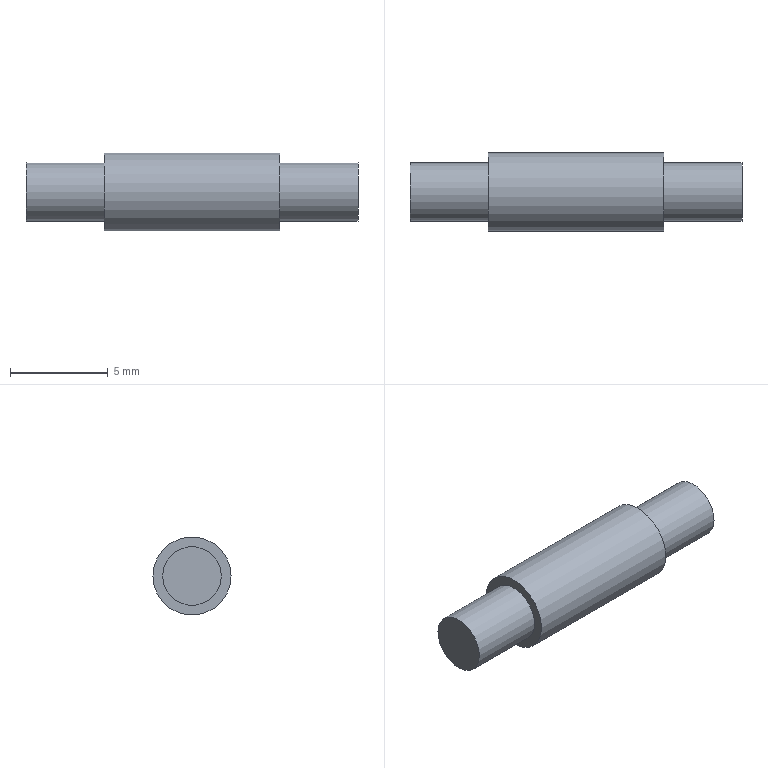Part | STEP file | 2-11.4 | 1 solid | 7 faces | box 17 x 4 x 4 mm | volume 169.646 mm3 | plane 4 | cylinder 3 | commonest cylinder face diameters 3 x2 4 x1
STEP:
#1=CARTESIAN_POINT('',(0.,0.,0.));
#2=DIRECTION('',(0.,0.,1.));
#3=DIRECTION('',(1.,0.,0.));
#4=AXIS2_PLACEMENT_3D('',#1,#2,#3);
#5=CARTESIAN_POINT('',(4.5,2.,0.));
#6=VERTEX_POINT('',#5);
#7=CARTESIAN_POINT('',(-4.5,2.,0.));
#8=VERTEX_POINT('',#7);
#9=CARTESIAN_POINT('',(4.5,2.,0.));
#10=DIRECTION('',(-1.,0.,0.));
#11=VECTOR('',#10,1.);
#12=LINE('',#9,#11);
#13=CARTESIAN_POINT('',(4.5,0.,0.));
#14=DIRECTION('',(-1.,0.,0.));
#15=DIRECTION('',(0.,1.,0.));
#16=AXIS2_PLACEMENT_3D('',#13,#14,#15);
#17=CYLINDRICAL_SURFACE('',#16,2.);
#18=CARTESIAN_POINT('',(6.283,0.));
#19=DIRECTION('',(0.,1.));
#20=VECTOR('',#19,1.);
#21=LINE('',#18,#20);
#22=(GEOMETRIC_REPRESENTATION_CONTEXT(2)PARAMETRIC_REPRESENTATION_CONTEXT()REPRESENTATION_CONTEXT('',''));
#23=DEFINITIONAL_REPRESENTATION('',(#21),#22);
#24=PCURVE('',#17,#23);
#25=CARTESIAN_POINT('',(0.,0.));
#26=DIRECTION('',(0.,1.));
#27=VECTOR('',#26,1.);
#28=LINE('',#25,#27);
#29=(GEOMETRIC_REPRESENTATION_CONTEXT(2)PARAMETRIC_REPRESENTATION_CONTEXT()REPRESENTATION_CONTEXT('',''));
#30=DEFINITIONAL_REPRESENTATION('',(#28),#29);
#31=PCURVE('',#17,#30);
#32=SEAM_CURVE('',#12,(#24,#31),.PCURVE_S1.);
#33=EDGE_CURVE('',#6,#8,#32,.T.);
#34=ORIENTED_EDGE('',*,*,#33,.T.);
#35=CARTESIAN_POINT('',(-4.5,0.,0.));
#36=DIRECTION('',(1.,0.,0.));
#37=DIRECTION('',(0.,1.,0.));
#38=AXIS2_PLACEMENT_3D('',#35,#36,#37);
#39=CIRCLE('',#38,2.);
#40=CARTESIAN_POINT('',(6.283,9.));
#41=DIRECTION('',(-1.,0.));
#42=VECTOR('',#41,1.);
#43=LINE('',#40,#42);
#44=(GEOMETRIC_REPRESENTATION_CONTEXT(2)PARAMETRIC_REPRESENTATION_CONTEXT()REPRESENTATION_CONTEXT('',''));
#45=DEFINITIONAL_REPRESENTATION('',(#43),#44);
#46=PCURVE('',#17,#45);
#47=CARTESIAN_POINT('',(-4.5,-0.5359,0.));
#48=DIRECTION('',(1.,0.,0.));
#49=DIRECTION('',(0.,0.,-1.));
#50=AXIS2_PLACEMENT_3D('',#47,#48,#49);
#51=PLANE('',#50);
#52=CARTESIAN_POINT('',(0.,0.5359));
#53=DIRECTION('',(0.,1.));
#54=AXIS2_PLACEMENT_2D('',#52,#53);
#55=CIRCLE('',#54,2.);
#56=(GEOMETRIC_REPRESENTATION_CONTEXT(2)PARAMETRIC_REPRESENTATION_CONTEXT()REPRESENTATION_CONTEXT('',''));
#57=DEFINITIONAL_REPRESENTATION('',(#55),#56);
#58=PCURVE('',#51,#57);
#59=SURFACE_CURVE('',#39,(#46,#58),.PCURVE_S1.);
#60=EDGE_CURVE('',#8,#8,#59,.T.);
#61=ORIENTED_EDGE('',*,*,#60,.T.);
#62=ORIENTED_EDGE('',*,*,#33,.F.);
#63=CARTESIAN_POINT('',(4.5,0.,0.));
#64=DIRECTION('',(1.,0.,0.));
#65=DIRECTION('',(0.,1.,0.));
#66=AXIS2_PLACEMENT_3D('',#63,#64,#65);
#67=CIRCLE('',#66,2.);
#68=CARTESIAN_POINT('',(6.283,0.));
#69=DIRECTION('',(-1.,0.));
#70=VECTOR('',#69,1.);
#71=LINE('',#68,#70);
#72=(GEOMETRIC_REPRESENTATION_CONTEXT(2)PARAMETRIC_REPRESENTATION_CONTEXT()REPRESENTATION_CONTEXT('',''));
#73=DEFINITIONAL_REPRESENTATION('',(#71),#72);
#74=PCURVE('',#17,#73);
#75=CARTESIAN_POINT('',(4.5,-0.5359,0.));
#76=DIRECTION('',(1.,0.,0.));
#77=DIRECTION('',(0.,0.,-1.));
#78=AXIS2_PLACEMENT_3D('',#75,#76,#77);
#79=PLANE('',#78);
#80=CARTESIAN_POINT('',(0.,0.5359));
#81=DIRECTION('',(0.,1.));
#82=AXIS2_PLACEMENT_2D('',#80,#81);
#83=CIRCLE('',#82,2.);
#84=(GEOMETRIC_REPRESENTATION_CONTEXT(2)PARAMETRIC_REPRESENTATION_CONTEXT()REPRESENTATION_CONTEXT('',''));
#85=DEFINITIONAL_REPRESENTATION('',(#83),#84);
#86=PCURVE('',#79,#85);
#87=SURFACE_CURVE('',#67,(#74,#86),.PCURVE_S1.);
#88=EDGE_CURVE('',#6,#6,#87,.T.);
#89=ORIENTED_EDGE('',*,*,#88,.F.);
#90=EDGE_LOOP('',(#34,#61,#62,#89));
#91=FACE_BOUND('',#90,.T.);
#92=ADVANCED_FACE('',(#91),#17,.T.);
#93=ORIENTED_EDGE('',*,*,#60,.T.);
#94=EDGE_LOOP('',(#93));
#95=FACE_BOUND('',#94,.F.);
#96=CARTESIAN_POINT('',(-4.5,1.5,0.));
#97=VERTEX_POINT('',#96);
#98=CARTESIAN_POINT('',(-4.5,0.,0.));
#99=DIRECTION('',(1.,0.,0.));
#100=DIRECTION('',(0.,1.,0.));
#101=AXIS2_PLACEMENT_3D('',#98,#99,#100);
#102=CIRCLE('',#101,1.5);
#103=CARTESIAN_POINT('',(0.,0.5359));
#104=DIRECTION('',(0.,1.));
#105=AXIS2_PLACEMENT_2D('',#103,#104);
#106=CIRCLE('',#105,1.5);
#107=(GEOMETRIC_REPRESENTATION_CONTEXT(2)PARAMETRIC_REPRESENTATION_CONTEXT()REPRESENTATION_CONTEXT('',''));
#108=DEFINITIONAL_REPRESENTATION('',(#106),#107);
#109=PCURVE('',#51,#108);
#110=CARTESIAN_POINT('',(-4.5,0.,0.));
#111=DIRECTION('',(-1.,0.,0.));
#112=DIRECTION('',(0.,1.,0.));
#113=AXIS2_PLACEMENT_3D('',#110,#111,#112);
#114=CYLINDRICAL_SURFACE('',#113,1.5);
#115=CARTESIAN_POINT('',(6.283,0.));
#116=DIRECTION('',(-1.,0.));
#117=VECTOR('',#116,1.);
#118=LINE('',#115,#117);
#119=(GEOMETRIC_REPRESENTATION_CONTEXT(2)PARAMETRIC_REPRESENTATION_CONTEXT()REPRESENTATION_CONTEXT('',''));
#120=DEFINITIONAL_REPRESENTATION('',(#118),#119);
#121=PCURVE('',#114,#120);
#122=SURFACE_CURVE('',#102,(#109,#121),.PCURVE_S1.);
#123=EDGE_CURVE('',#97,#97,#122,.T.);
#124=ORIENTED_EDGE('',*,*,#123,.F.);
#125=EDGE_LOOP('',(#124));
#126=FACE_BOUND('',#125,.F.);
#127=ADVANCED_FACE('',(#95,#126),#51,.F.);
#128=CARTESIAN_POINT('',(-8.5,1.5,0.));
#129=VERTEX_POINT('',#128);
#130=CARTESIAN_POINT('',(-4.5,1.5,0.));
#131=DIRECTION('',(-1.,0.,0.));
#132=VECTOR('',#131,1.);
#133=LINE('',#130,#132);
#134=CARTESIAN_POINT('',(6.283,0.));
#135=DIRECTION('',(0.,1.));
#136=VECTOR('',#135,1.);
#137=LINE('',#134,#136);
#138=(GEOMETRIC_REPRESENTATION_CONTEXT(2)PARAMETRIC_REPRESENTATION_CONTEXT()REPRESENTATION_CONTEXT('',''));
#139=DEFINITIONAL_REPRESENTATION('',(#137),#138);
#140=PCURVE('',#114,#139);
#141=CARTESIAN_POINT('',(0.,0.));
#142=DIRECTION('',(0.,1.));
#143=VECTOR('',#142,1.);
#144=LINE('',#141,#143);
#145=(GEOMETRIC_REPRESENTATION_CONTEXT(2)PARAMETRIC_REPRESENTATION_CONTEXT()REPRESENTATION_CONTEXT('',''));
#146=DEFINITIONAL_REPRESENTATION('',(#144),#145);
#147=PCURVE('',#114,#146);
#148=SEAM_CURVE('',#133,(#140,#147),.PCURVE_S1.);
#149=EDGE_CURVE('',#97,#129,#148,.T.);
#150=ORIENTED_EDGE('',*,*,#149,.T.);
#151=CARTESIAN_POINT('',(-8.5,0.,0.));
#152=DIRECTION('',(1.,0.,0.));
#153=DIRECTION('',(0.,1.,0.));
#154=AXIS2_PLACEMENT_3D('',#151,#152,#153);
#155=CIRCLE('',#154,1.5);
#156=CARTESIAN_POINT('',(6.283,4.));
#157=DIRECTION('',(-1.,0.));
#158=VECTOR('',#157,1.);
#159=LINE('',#156,#158);
#160=(GEOMETRIC_REPRESENTATION_CONTEXT(2)PARAMETRIC_REPRESENTATION_CONTEXT()REPRESENTATION_CONTEXT('',''));
#161=DEFINITIONAL_REPRESENTATION('',(#159),#160);
#162=PCURVE('',#114,#161);
#163=CARTESIAN_POINT('',(-8.5,-0.4019,0.));
#164=DIRECTION('',(1.,0.,0.));
#165=DIRECTION('',(0.,0.,-1.));
#166=AXIS2_PLACEMENT_3D('',#163,#164,#165);
#167=PLANE('',#166);
#168=CARTESIAN_POINT('',(0.,0.4019));
#169=DIRECTION('',(0.,1.));
#170=AXIS2_PLACEMENT_2D('',#168,#169);
#171=CIRCLE('',#170,1.5);
#172=(GEOMETRIC_REPRESENTATION_CONTEXT(2)PARAMETRIC_REPRESENTATION_CONTEXT()REPRESENTATION_CONTEXT('',''));
#173=DEFINITIONAL_REPRESENTATION('',(#171),#172);
#174=PCURVE('',#167,#173);
#175=SURFACE_CURVE('',#155,(#162,#174),.PCURVE_S1.);
#176=EDGE_CURVE('',#129,#129,#175,.T.);
#177=ORIENTED_EDGE('',*,*,#176,.T.);
#178=ORIENTED_EDGE('',*,*,#149,.F.);
#179=ORIENTED_EDGE('',*,*,#123,.F.);
#180=EDGE_LOOP('',(#150,#177,#178,#179));
#181=FACE_BOUND('',#180,.T.);
#182=ADVANCED_FACE('',(#181),#114,.T.);
#183=ORIENTED_EDGE('',*,*,#176,.T.);
#184=EDGE_LOOP('',(#183));
#185=FACE_BOUND('',#184,.F.);
#186=ADVANCED_FACE('',(#185),#167,.F.);
#187=ORIENTED_EDGE('',*,*,#88,.T.);
#188=EDGE_LOOP('',(#187));
#189=FACE_BOUND('',#188,.T.);
#190=CARTESIAN_POINT('',(4.5,1.5,0.));
#191=VERTEX_POINT('',#190);
#192=CARTESIAN_POINT('',(4.5,0.,0.));
#193=DIRECTION('',(1.,0.,0.));
#194=DIRECTION('',(0.,1.,0.));
#195=AXIS2_PLACEMENT_3D('',#192,#193,#194);
#196=CIRCLE('',#195,1.5);
#197=CARTESIAN_POINT('',(0.,0.5359));
#198=DIRECTION('',(0.,1.));
#199=AXIS2_PLACEMENT_2D('',#197,#198);
#200=CIRCLE('',#199,1.5);
#201=(GEOMETRIC_REPRESENTATION_CONTEXT(2)PARAMETRIC_REPRESENTATION_CONTEXT()REPRESENTATION_CONTEXT('',''));
#202=DEFINITIONAL_REPRESENTATION('',(#200),#201);
#203=PCURVE('',#79,#202);
#204=CARTESIAN_POINT('',(4.5,0.,0.));
#205=DIRECTION('',(1.,0.,0.));
#206=DIRECTION('',(0.,1.,0.));
#207=AXIS2_PLACEMENT_3D('',#204,#205,#206);
#208=CYLINDRICAL_SURFACE('',#207,1.5);
#209=CARTESIAN_POINT('',(0.,0.));
#210=DIRECTION('',(1.,0.));
#211=VECTOR('',#210,1.);
#212=LINE('',#209,#211);
#213=(GEOMETRIC_REPRESENTATION_CONTEXT(2)PARAMETRIC_REPRESENTATION_CONTEXT()REPRESENTATION_CONTEXT('',''));
#214=DEFINITIONAL_REPRESENTATION('',(#212),#213);
#215=PCURVE('',#208,#214);
#216=SURFACE_CURVE('',#196,(#203,#215),.PCURVE_S1.);
#217=EDGE_CURVE('',#191,#191,#216,.T.);
#218=ORIENTED_EDGE('',*,*,#217,.F.);
#219=EDGE_LOOP('',(#218));
#220=FACE_BOUND('',#219,.T.);
#221=ADVANCED_FACE('',(#189,#220),#79,.T.);
#222=ORIENTED_EDGE('',*,*,#217,.T.);
#223=CARTESIAN_POINT('',(8.5,1.5,0.));
#224=VERTEX_POINT('',#223);
#225=CARTESIAN_POINT('',(4.5,1.5,0.));
#226=DIRECTION('',(1.,0.,0.));
#227=VECTOR('',#226,1.);
#228=LINE('',#225,#227);
#229=CARTESIAN_POINT('',(6.283,0.));
#230=DIRECTION('',(0.,1.));
#231=VECTOR('',#230,1.);
#232=LINE('',#229,#231);
#233=(GEOMETRIC_REPRESENTATION_CONTEXT(2)PARAMETRIC_REPRESENTATION_CONTEXT()REPRESENTATION_CONTEXT('',''));
#234=DEFINITIONAL_REPRESENTATION('',(#232),#233);
#235=PCURVE('',#208,#234);
#236=CARTESIAN_POINT('',(0.,0.));
#237=DIRECTION('',(0.,1.));
#238=VECTOR('',#237,1.);
#239=LINE('',#236,#238);
#240=(GEOMETRIC_REPRESENTATION_CONTEXT(2)PARAMETRIC_REPRESENTATION_CONTEXT()REPRESENTATION_CONTEXT('',''));
#241=DEFINITIONAL_REPRESENTATION('',(#239),#240);
#242=PCURVE('',#208,#241);
#243=SEAM_CURVE('',#228,(#235,#242),.PCURVE_S1.);
#244=EDGE_CURVE('',#191,#224,#243,.T.);
#245=ORIENTED_EDGE('',*,*,#244,.T.);
#246=CARTESIAN_POINT('',(8.5,0.,0.));
#247=DIRECTION('',(1.,0.,0.));
#248=DIRECTION('',(0.,1.,0.));
#249=AXIS2_PLACEMENT_3D('',#246,#247,#248);
#250=CIRCLE('',#249,1.5);
#251=CARTESIAN_POINT('',(0.,4.));
#252=DIRECTION('',(1.,0.));
#253=VECTOR('',#252,1.);
#254=LINE('',#251,#253);
#255=(GEOMETRIC_REPRESENTATION_CONTEXT(2)PARAMETRIC_REPRESENTATION_CONTEXT()REPRESENTATION_CONTEXT('',''));
#256=DEFINITIONAL_REPRESENTATION('',(#254),#255);
#257=PCURVE('',#208,#256);
#258=CARTESIAN_POINT('',(8.5,-0.4019,0.));
#259=DIRECTION('',(1.,0.,0.));
#260=DIRECTION('',(0.,0.,-1.));
#261=AXIS2_PLACEMENT_3D('',#258,#259,#260);
#262=PLANE('',#261);
#263=CARTESIAN_POINT('',(0.,0.4019));
#264=DIRECTION('',(0.,1.));
#265=AXIS2_PLACEMENT_2D('',#263,#264);
#266=CIRCLE('',#265,1.5);
#267=(GEOMETRIC_REPRESENTATION_CONTEXT(2)PARAMETRIC_REPRESENTATION_CONTEXT()REPRESENTATION_CONTEXT('',''));
#268=DEFINITIONAL_REPRESENTATION('',(#266),#267);
#269=PCURVE('',#262,#268);
#270=SURFACE_CURVE('',#250,(#257,#269),.PCURVE_S1.);
#271=EDGE_CURVE('',#224,#224,#270,.T.);
#272=ORIENTED_EDGE('',*,*,#271,.F.);
#273=ORIENTED_EDGE('',*,*,#244,.F.);
#274=EDGE_LOOP('',(#222,#245,#272,#273));
#275=FACE_BOUND('',#274,.T.);
#276=ADVANCED_FACE('',(#275),#208,.T.);
#277=ORIENTED_EDGE('',*,*,#271,.T.);
#278=EDGE_LOOP('',(#277));
#279=FACE_BOUND('',#278,.T.);
#280=ADVANCED_FACE('',(#279),#262,.T.);
#281=CLOSED_SHELL('',(#92,#127,#182,#186,#221,#276,#280));
#282=MANIFOLD_SOLID_BREP('',#281);
#283=(LENGTH_UNIT()NAMED_UNIT(*)SI_UNIT(.MILLI.,.METRE.));
#284=UNCERTAINTY_MEASURE_WITH_UNIT(LENGTH_MEASURE(0.0000001),#283,'','');
#285=(NAMED_UNIT(*)PLANE_ANGLE_UNIT()SI_UNIT($,.RADIAN.));
#286=(NAMED_UNIT(*)SI_UNIT($,.STERADIAN.)SOLID_ANGLE_UNIT());
#287=(GEOMETRIC_REPRESENTATION_CONTEXT(3)GLOBAL_UNCERTAINTY_ASSIGNED_CONTEXT((#284))GLOBAL_UNIT_ASSIGNED_CONTEXT((#283,#285,#286))REPRESENTATION_CONTEXT('',''));
#288=ADVANCED_BREP_SHAPE_REPRESENTATION('',(#4,#282),#287);